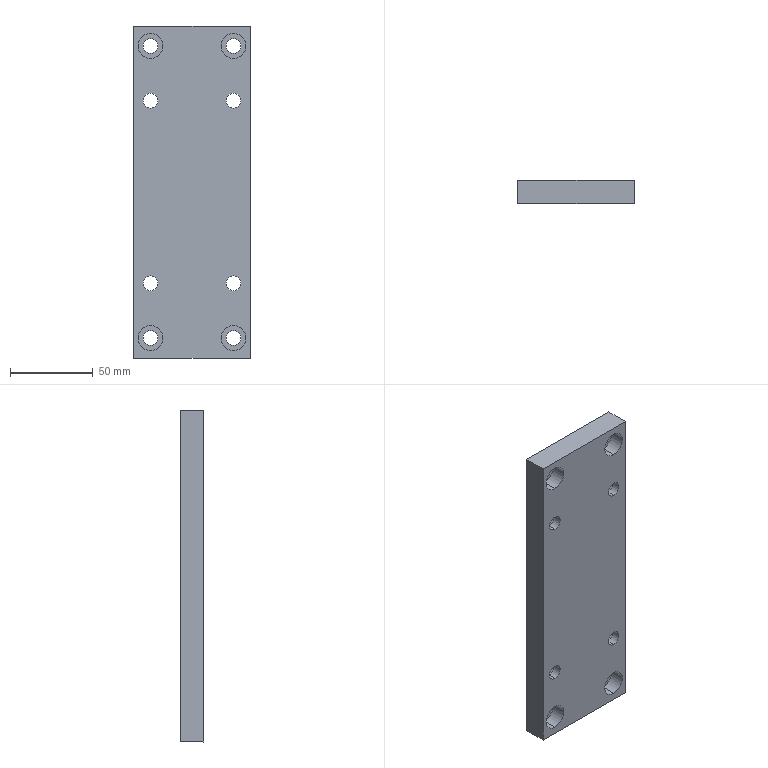Part | SolidWorks | features HoleWzd 2, Extrusion 1 | 1 solid | 46 faces | box 70 x 14 x 200 mm | volume 180732 mm3 | cylinder 32 | plane 14 | commonest cylinder face diameters 9 x16 15 x16
STEP:
#1=CARTESIAN_POINT('',(60.,9.,-180.5));
#2=VERTEX_POINT('',#1);
#3=CARTESIAN_POINT('',(60.,9.,-195.5));
#4=VERTEX_POINT('',#3);
#5=CARTESIAN_POINT('',(60.,9.,-188.));
#6=DIRECTION('',(0.,-1.,0.));
#7=DIRECTION('',(0.,0.,-1.));
#8=AXIS2_PLACEMENT_3D('',#5,#6,#7);
#9=CIRCLE('',#8,7.5);
#10=EDGE_CURVE('',#2,#4,#9,.T.);
#11=ORIENTED_EDGE('',*,*,#10,.F.);
#12=CARTESIAN_POINT('',(60.,0.,-180.5));
#13=VERTEX_POINT('',#12);
#14=CARTESIAN_POINT('',(60.,0.,-180.5));
#15=DIRECTION('',(0.,-1.,0.));
#16=VECTOR('',#15,1000.);
#17=LINE('',#14,#16);
#18=EDGE_CURVE('',#2,#13,#17,.T.);
#19=ORIENTED_EDGE('',*,*,#18,.T.);
#20=CARTESIAN_POINT('',(60.,0.,-195.5));
#21=VERTEX_POINT('',#20);
#22=CARTESIAN_POINT('',(60.,0.,-188.));
#23=DIRECTION('',(0.,-1.,0.));
#24=DIRECTION('',(0.,0.,-1.));
#25=AXIS2_PLACEMENT_3D('',#22,#23,#24);
#26=CIRCLE('',#25,7.5);
#27=EDGE_CURVE('',#13,#21,#26,.T.);
#28=ORIENTED_EDGE('',*,*,#27,.T.);
#29=CARTESIAN_POINT('',(60.,0.,-195.5));
#30=DIRECTION('',(0.,-1.,0.));
#31=VECTOR('',#30,1000.);
#32=LINE('',#29,#31);
#33=EDGE_CURVE('',#4,#21,#32,.T.);
#34=ORIENTED_EDGE('',*,*,#33,.F.);
#35=EDGE_LOOP('',(#11,#19,#28,#34));
#36=FACE_OUTER_BOUND('',#35,.T.);
#37=CARTESIAN_POINT('',(60.,0.,-188.));
#38=DIRECTION('',(0.,-1.,0.));
#39=DIRECTION('',(0.,0.,-1.));
#40=AXIS2_PLACEMENT_3D('',#37,#38,#39);
#41=CYLINDRICAL_SURFACE('',#40,7.5);
#42=ADVANCED_FACE('',(#36),#41,.F.);
#43=CARTESIAN_POINT('',(60.,14.,-183.5));
#44=VERTEX_POINT('',#43);
#45=CARTESIAN_POINT('',(60.,14.,-192.5));
#46=VERTEX_POINT('',#45);
#47=CARTESIAN_POINT('',(60.,14.,-188.));
#48=DIRECTION('',(0.,-1.,0.));
#49=DIRECTION('',(0.,0.,-1.));
#50=AXIS2_PLACEMENT_3D('',#47,#48,#49);
#51=CIRCLE('',#50,4.5);
#52=EDGE_CURVE('',#44,#46,#51,.T.);
#53=ORIENTED_EDGE('',*,*,#52,.F.);
#54=CARTESIAN_POINT('',(60.,9.,-183.5));
#55=VERTEX_POINT('',#54);
#56=CARTESIAN_POINT('',(60.,0.,-183.5));
#57=DIRECTION('',(0.,-1.,0.));
#58=VECTOR('',#57,1000.);
#59=LINE('',#56,#58);
#60=EDGE_CURVE('',#44,#55,#59,.T.);
#61=ORIENTED_EDGE('',*,*,#60,.T.);
#62=CARTESIAN_POINT('',(60.,9.,-192.5));
#63=VERTEX_POINT('',#62);
#64=CARTESIAN_POINT('',(60.,9.,-188.));
#65=DIRECTION('',(0.,-1.,0.));
#66=DIRECTION('',(0.,0.,-1.));
#67=AXIS2_PLACEMENT_3D('',#64,#65,#66);
#68=CIRCLE('',#67,4.5);
#69=EDGE_CURVE('',#55,#63,#68,.T.);
#70=ORIENTED_EDGE('',*,*,#69,.T.);
#71=CARTESIAN_POINT('',(60.,0.,-192.5));
#72=DIRECTION('',(0.,-1.,0.));
#73=VECTOR('',#72,1000.);
#74=LINE('',#71,#73);
#75=EDGE_CURVE('',#46,#63,#74,.T.);
#76=ORIENTED_EDGE('',*,*,#75,.F.);
#77=EDGE_LOOP('',(#53,#61,#70,#76));
#78=FACE_OUTER_BOUND('',#77,.T.);
#79=CARTESIAN_POINT('',(60.,0.,-188.));
#80=DIRECTION('',(0.,-1.,0.));
#81=DIRECTION('',(0.,0.,-1.));
#82=AXIS2_PLACEMENT_3D('',#79,#80,#81);
#83=CYLINDRICAL_SURFACE('',#82,4.5);
#84=ADVANCED_FACE('',(#78),#83,.F.);
#85=CARTESIAN_POINT('',(10.,9.,-180.5));
#86=VERTEX_POINT('',#85);
#87=CARTESIAN_POINT('',(10.,9.,-195.5));
#88=VERTEX_POINT('',#87);
#89=CARTESIAN_POINT('',(10.,9.,-188.));
#90=DIRECTION('',(0.,-1.,0.));
#91=DIRECTION('',(0.,0.,-1.));
#92=AXIS2_PLACEMENT_3D('',#89,#90,#91);
#93=CIRCLE('',#92,7.5);
#94=EDGE_CURVE('',#86,#88,#93,.T.);
#95=ORIENTED_EDGE('',*,*,#94,.F.);
#96=CARTESIAN_POINT('',(10.,0.,-180.5));
#97=VERTEX_POINT('',#96);
#98=CARTESIAN_POINT('',(10.,0.,-180.5));
#99=DIRECTION('',(0.,-1.,0.));
#100=VECTOR('',#99,1000.);
#101=LINE('',#98,#100);
#102=EDGE_CURVE('',#86,#97,#101,.T.);
#103=ORIENTED_EDGE('',*,*,#102,.T.);
#104=CARTESIAN_POINT('',(10.,0.,-195.5));
#105=VERTEX_POINT('',#104);
#106=CARTESIAN_POINT('',(10.,0.,-188.));
#107=DIRECTION('',(0.,-1.,0.));
#108=DIRECTION('',(0.,0.,-1.));
#109=AXIS2_PLACEMENT_3D('',#106,#107,#108);
#110=CIRCLE('',#109,7.5);
#111=EDGE_CURVE('',#97,#105,#110,.T.);
#112=ORIENTED_EDGE('',*,*,#111,.T.);
#113=CARTESIAN_POINT('',(10.,0.,-195.5));
#114=DIRECTION('',(0.,-1.,0.));
#115=VECTOR('',#114,1000.);
#116=LINE('',#113,#115);
#117=EDGE_CURVE('',#88,#105,#116,.T.);
#118=ORIENTED_EDGE('',*,*,#117,.F.);
#119=EDGE_LOOP('',(#95,#103,#112,#118));
#120=FACE_OUTER_BOUND('',#119,.T.);
#121=CARTESIAN_POINT('',(10.,0.,-188.));
#122=DIRECTION('',(0.,-1.,0.));
#123=DIRECTION('',(0.,0.,-1.));
#124=AXIS2_PLACEMENT_3D('',#121,#122,#123);
#125=CYLINDRICAL_SURFACE('',#124,7.5);
#126=ADVANCED_FACE('',(#120),#125,.F.);
#127=CARTESIAN_POINT('',(10.,14.,-183.5));
#128=VERTEX_POINT('',#127);
#129=CARTESIAN_POINT('',(10.,14.,-192.5));
#130=VERTEX_POINT('',#129);
#131=CARTESIAN_POINT('',(10.,14.,-188.));
#132=DIRECTION('',(0.,-1.,0.));
#133=DIRECTION('',(0.,0.,-1.));
#134=AXIS2_PLACEMENT_3D('',#131,#132,#133);
#135=CIRCLE('',#134,4.5);
#136=EDGE_CURVE('',#128,#130,#135,.T.);
#137=ORIENTED_EDGE('',*,*,#136,.F.);
#138=CARTESIAN_POINT('',(10.,9.,-183.5));
#139=VERTEX_POINT('',#138);
#140=CARTESIAN_POINT('',(10.,0.,-183.5));
#141=DIRECTION('',(0.,-1.,0.));
#142=VECTOR('',#141,1000.);
#143=LINE('',#140,#142);
#144=EDGE_CURVE('',#128,#139,#143,.T.);
#145=ORIENTED_EDGE('',*,*,#144,.T.);
#146=CARTESIAN_POINT('',(10.,9.,-192.5));
#147=VERTEX_POINT('',#146);
#148=CARTESIAN_POINT('',(10.,9.,-188.));
#149=DIRECTION('',(0.,-1.,0.));
#150=DIRECTION('',(0.,0.,-1.));
#151=AXIS2_PLACEMENT_3D('',#148,#149,#150);
#152=CIRCLE('',#151,4.5);
#153=EDGE_CURVE('',#139,#147,#152,.T.);
#154=ORIENTED_EDGE('',*,*,#153,.T.);
#155=CARTESIAN_POINT('',(10.,0.,-192.5));
#156=DIRECTION('',(0.,-1.,0.));
#157=VECTOR('',#156,1000.);
#158=LINE('',#155,#157);
#159=EDGE_CURVE('',#130,#147,#158,.T.);
#160=ORIENTED_EDGE('',*,*,#159,.F.);
#161=EDGE_LOOP('',(#137,#145,#154,#160));
#162=FACE_OUTER_BOUND('',#161,.T.);
#163=CARTESIAN_POINT('',(10.,0.,-188.));
#164=DIRECTION('',(0.,-1.,0.));
#165=DIRECTION('',(0.,0.,-1.));
#166=AXIS2_PLACEMENT_3D('',#163,#164,#165);
#167=CYLINDRICAL_SURFACE('',#166,4.5);
#168=ADVANCED_FACE('',(#162),#167,.F.);
#169=CARTESIAN_POINT('',(10.,9.,-4.5));
#170=VERTEX_POINT('',#169);
#171=CARTESIAN_POINT('',(10.,9.,-19.5));
#172=VERTEX_POINT('',#171);
#173=CARTESIAN_POINT('',(10.,9.,-12.));
#174=DIRECTION('',(0.,-1.,0.));
#175=DIRECTION('',(0.,0.,-1.));
#176=AXIS2_PLACEMENT_3D('',#173,#174,#175);
#177=CIRCLE('',#176,7.5);
#178=EDGE_CURVE('',#170,#172,#177,.T.);
#179=ORIENTED_EDGE('',*,*,#178,.F.);
#180=CARTESIAN_POINT('',(10.,0.,-4.5));
#181=VERTEX_POINT('',#180);
#182=CARTESIAN_POINT('',(10.,0.,-4.5));
#183=DIRECTION('',(0.,-1.,0.));
#184=VECTOR('',#183,1000.);
#185=LINE('',#182,#184);
#186=EDGE_CURVE('',#170,#181,#185,.T.);
#187=ORIENTED_EDGE('',*,*,#186,.T.);
#188=CARTESIAN_POINT('',(10.,0.,-19.5));
#189=VERTEX_POINT('',#188);
#190=CARTESIAN_POINT('',(10.,0.,-12.));
#191=DIRECTION('',(0.,-1.,0.));
#192=DIRECTION('',(0.,0.,-1.));
#193=AXIS2_PLACEMENT_3D('',#190,#191,#192);
#194=CIRCLE('',#193,7.5);
#195=EDGE_CURVE('',#181,#189,#194,.T.);
#196=ORIENTED_EDGE('',*,*,#195,.T.);
#197=CARTESIAN_POINT('',(10.,0.,-19.5));
#198=DIRECTION('',(0.,-1.,0.));
#199=VECTOR('',#198,1000.);
#200=LINE('',#197,#199);
#201=EDGE_CURVE('',#172,#189,#200,.T.);
#202=ORIENTED_EDGE('',*,*,#201,.F.);
#203=EDGE_LOOP('',(#179,#187,#196,#202));
#204=FACE_OUTER_BOUND('',#203,.T.);
#205=CARTESIAN_POINT('',(10.,0.,-12.));
#206=DIRECTION('',(0.,-1.,0.));
#207=DIRECTION('',(0.,0.,-1.));
#208=AXIS2_PLACEMENT_3D('',#205,#206,#207);
#209=CYLINDRICAL_SURFACE('',#208,7.5);
#210=ADVANCED_FACE('',(#204),#209,.F.);
#211=CARTESIAN_POINT('',(10.,14.,-7.5));
#212=VERTEX_POINT('',#211);
#213=CARTESIAN_POINT('',(10.,14.,-16.5));
#214=VERTEX_POINT('',#213);
#215=CARTESIAN_POINT('',(10.,14.,-12.));
#216=DIRECTION('',(0.,-1.,0.));
#217=DIRECTION('',(0.,0.,-1.));
#218=AXIS2_PLACEMENT_3D('',#215,#216,#217);
#219=CIRCLE('',#218,4.5);
#220=EDGE_CURVE('',#212,#214,#219,.T.);
#221=ORIENTED_EDGE('',*,*,#220,.F.);
#222=CARTESIAN_POINT('',(10.,9.,-7.5));
#223=VERTEX_POINT('',#222);
#224=CARTESIAN_POINT('',(10.,0.,-7.5));
#225=DIRECTION('',(0.,-1.,0.));
#226=VECTOR('',#225,1000.);
#227=LINE('',#224,#226);
#228=EDGE_CURVE('',#212,#223,#227,.T.);
#229=ORIENTED_EDGE('',*,*,#228,.T.);
#230=CARTESIAN_POINT('',(10.,9.,-16.5));
#231=VERTEX_POINT('',#230);
#232=CARTESIAN_POINT('',(10.,9.,-12.));
#233=DIRECTION('',(0.,-1.,0.));
#234=DIRECTION('',(0.,0.,-1.));
#235=AXIS2_PLACEMENT_3D('',#232,#233,#234);
#236=CIRCLE('',#235,4.5);
#237=EDGE_CURVE('',#223,#231,#236,.T.);
#238=ORIENTED_EDGE('',*,*,#237,.T.);
#239=CARTESIAN_POINT('',(10.,0.,-16.5));
#240=DIRECTION('',(0.,-1.,0.));
#241=VECTOR('',#240,1000.);
#242=LINE('',#239,#241);
#243=EDGE_CURVE('',#214,#231,#242,.T.);
#244=ORIENTED_EDGE('',*,*,#243,.F.);
#245=EDGE_LOOP('',(#221,#229,#238,#244));
#246=FACE_OUTER_BOUND('',#245,.T.);
#247=CARTESIAN_POINT('',(10.,0.,-12.));
#248=DIRECTION('',(0.,-1.,0.));
#249=DIRECTION('',(0.,0.,-1.));
#250=AXIS2_PLACEMENT_3D('',#247,#248,#249);
#251=CYLINDRICAL_SURFACE('',#250,4.5);
#252=ADVANCED_FACE('',(#246),#251,.F.);
#253=CARTESIAN_POINT('',(60.,9.,-4.5));
#254=VERTEX_POINT('',#253);
#255=CARTESIAN_POINT('',(60.,9.,-19.5));
#256=VERTEX_POINT('',#255);
#257=CARTESIAN_POINT('',(60.,9.,-12.));
#258=DIRECTION('',(0.,-1.,0.));
#259=DIRECTION('',(0.,0.,-1.));
#260=AXIS2_PLACEMENT_3D('',#257,#258,#259);
#261=CIRCLE('',#260,7.5);
#262=EDGE_CURVE('',#254,#256,#261,.T.);
#263=ORIENTED_EDGE('',*,*,#262,.F.);
#264=CARTESIAN_POINT('',(60.,0.,-4.5));
#265=VERTEX_POINT('',#264);
#266=CARTESIAN_POINT('',(60.,0.,-4.5));
#267=DIRECTION('',(0.,-1.,0.));
#268=VECTOR('',#267,1000.);
#269=LINE('',#266,#268);
#270=EDGE_CURVE('',#254,#265,#269,.T.);
#271=ORIENTED_EDGE('',*,*,#270,.T.);
#272=CARTESIAN_POINT('',(60.,0.,-19.5));
#273=VERTEX_POINT('',#272);
#274=CARTESIAN_POINT('',(60.,0.,-12.));
#275=DIRECTION('',(0.,-1.,0.));
#276=DIRECTION('',(0.,0.,-1.));
#277=AXIS2_PLACEMENT_3D('',#274,#275,#276);
#278=CIRCLE('',#277,7.5);
#279=EDGE_CURVE('',#265,#273,#278,.T.);
#280=ORIENTED_EDGE('',*,*,#279,.T.);
#281=CARTESIAN_POINT('',(60.,0.,-19.5));
#282=DIRECTION('',(0.,-1.,0.));
#283=VECTOR('',#282,1000.);
#284=LINE('',#281,#283);
#285=EDGE_CURVE('',#256,#273,#284,.T.);
#286=ORIENTED_EDGE('',*,*,#285,.F.);
#287=EDGE_LOOP('',(#263,#271,#280,#286));
#288=FACE_OUTER_BOUND('',#287,.T.);
#289=CARTESIAN_POINT('',(60.,0.,-12.));
#290=DIRECTION('',(0.,-1.,0.));
#291=DIRECTION('',(0.,0.,-1.));
#292=AXIS2_PLACEMENT_3D('',#289,#290,#291);
#293=CYLINDRICAL_SURFACE('',#292,7.5);
#294=ADVANCED_FACE('',(#288),#293,.F.);
#295=CARTESIAN_POINT('',(60.,14.,-7.5));
#296=VERTEX_POINT('',#295);
#297=CARTESIAN_POINT('',(60.,14.,-16.5));
#298=VERTEX_POINT('',#297);
#299=CARTESIAN_POINT('',(60.,14.,-12.));
#300=DIRECTION('',(0.,-1.,0.));
#301=DIRECTION('',(0.,0.,-1.));
#302=AXIS2_PLACEMENT_3D('',#299,#300,#301);
#303=CIRCLE('',#302,4.5);
#304=EDGE_CURVE('',#296,#298,#303,.T.);
#305=ORIENTED_EDGE('',*,*,#304,.F.);
#306=CARTESIAN_POINT('',(60.,9.,-7.5));
#307=VERTEX_POINT('',#306);
#308=CARTESIAN_POINT('',(60.,0.,-7.5));
#309=DIRECTION('',(0.,-1.,0.));
#310=VECTOR('',#309,1000.);
#311=LINE('',#308,#310);
#312=EDGE_CURVE('',#296,#307,#311,.T.);
#313=ORIENTED_EDGE('',*,*,#312,.T.);
#314=CARTESIAN_POINT('',(60.,9.,-16.5));
#315=VERTEX_POINT('',#314);
#316=CARTESIAN_POINT('',(60.,9.,-12.));
#317=DIRECTION('',(0.,-1.,0.));
#318=DIRECTION('',(0.,0.,-1.));
#319=AXIS2_PLACEMENT_3D('',#316,#317,#318);
#320=CIRCLE('',#319,4.5);
#321=EDGE_CURVE('',#307,#315,#320,.T.);
#322=ORIENTED_EDGE('',*,*,#321,.T.);
#323=CARTESIAN_POINT('',(60.,0.,-16.5));
#324=DIRECTION('',(0.,-1.,0.));
#325=VECTOR('',#324,1000.);
#326=LINE('',#323,#325);
#327=EDGE_CURVE('',#298,#315,#326,.T.);
#328=ORIENTED_EDGE('',*,*,#327,.F.);
#329=EDGE_LOOP('',(#305,#313,#322,#328));
#330=FACE_OUTER_BOUND('',#329,.T.);
#331=CARTESIAN_POINT('',(60.,0.,-12.));
#332=DIRECTION('',(0.,-1.,0.));
#333=DIRECTION('',(0.,0.,-1.));
#334=AXIS2_PLACEMENT_3D('',#331,#332,#333);
#335=CYLINDRICAL_SURFACE('',#334,4.5);
#336=ADVANCED_FACE('',(#330),#335,.F.);
#337=CARTESIAN_POINT('',(10.,5.,-162.5));
#338=VERTEX_POINT('',#337);
#339=CARTESIAN_POINT('',(10.,5.,-147.5));
#340=VERTEX_POINT('',#339);
#341=CARTESIAN_POINT('',(10.,5.,-155.));
#342=DIRECTION('',(0.,1.,0.));
#343=DIRECTION('',(0.,0.,1.));
#344=AXIS2_PLACEMENT_3D('',#341,#342,#343);
#345=CIRCLE('',#344,7.5);
#346=EDGE_CURVE('',#338,#340,#345,.T.);
#347=ORIENTED_EDGE('',*,*,#346,.F.);
#348=CARTESIAN_POINT('',(10.,14.,-162.5));
#349=VERTEX_POINT('',#348);
#350=CARTESIAN_POINT('',(10.,14.,-162.5));
#351=DIRECTION('',(0.,1.,0.));
#352=VECTOR('',#351,1000.);
#353=LINE('',#350,#352);
#354=EDGE_CURVE('',#338,#349,#353,.T.);
#355=ORIENTED_EDGE('',*,*,#354,.T.);
#356=CARTESIAN_POINT('',(10.,14.,-147.5));
#357=VERTEX_POINT('',#356);
#358=CARTESIAN_POINT('',(10.,14.,-155.));
#359=DIRECTION('',(0.,1.,0.));
#360=DIRECTION('',(0.,0.,1.));
#361=AXIS2_PLACEMENT_3D('',#358,#359,#360);
#362=CIRCLE('',#361,7.5);
#363=EDGE_CURVE('',#349,#357,#362,.T.);
#364=ORIENTED_EDGE('',*,*,#363,.T.);
#365=CARTESIAN_POINT('',(10.,14.,-147.5));
#366=DIRECTION('',(0.,1.,0.));
#367=VECTOR('',#366,1000.);
#368=LINE('',#365,#367);
#369=EDGE_CURVE('',#340,#357,#368,.T.);
#370=ORIENTED_EDGE('',*,*,#369,.F.);
#371=EDGE_LOOP('',(#347,#355,#364,#370));
#372=FACE_OUTER_BOUND('',#371,.T.);
#373=CARTESIAN_POINT('',(10.,14.,-155.));
#374=DIRECTION('',(0.,1.,0.));
#375=DIRECTION('',(0.,0.,1.));
#376=AXIS2_PLACEMENT_3D('',#373,#374,#375);
#377=CYLINDRICAL_SURFACE('',#376,7.5);
#378=ADVANCED_FACE('',(#372),#377,.F.);
#379=CARTESIAN_POINT('',(10.,0.,-159.5));
#380=VERTEX_POINT('',#379);
#381=CARTESIAN_POINT('',(10.,0.,-150.5));
#382=VERTEX_POINT('',#381);
#383=CARTESIAN_POINT('',(10.,0.,-155.));
#384=DIRECTION('',(0.,1.,0.));
#385=DIRECTION('',(0.,0.,1.));
#386=AXIS2_PLACEMENT_3D('',#383,#384,#385);
#387=CIRCLE('',#386,4.5);
#388=EDGE_CURVE('',#380,#382,#387,.T.);
#389=ORIENTED_EDGE('',*,*,#388,.F.);
#390=CARTESIAN_POINT('',(10.,5.,-159.5));
#391=VERTEX_POINT('',#390);
#392=CARTESIAN_POINT('',(10.,14.,-159.5));
#393=DIRECTION('',(0.,1.,0.));
#394=VECTOR('',#393,1000.);
#395=LINE('',#392,#394);
#396=EDGE_CURVE('',#380,#391,#395,.T.);
#397=ORIENTED_EDGE('',*,*,#396,.T.);
#398=CARTESIAN_POINT('',(10.,5.,-150.5));
#399=VERTEX_POINT('',#398);
#400=CARTESIAN_POINT('',(10.,5.,-155.));
#401=DIRECTION('',(0.,1.,0.));
#402=DIRECTION('',(0.,0.,1.));
#403=AXIS2_PLACEMENT_3D('',#400,#401,#402);
#404=CIRCLE('',#403,4.5);
#405=EDGE_CURVE('',#391,#399,#404,.T.);
#406=ORIENTED_EDGE('',*,*,#405,.T.);
#407=CARTESIAN_POINT('',(10.,14.,-150.5));
#408=DIRECTION('',(0.,1.,0.));
#409=VECTOR('',#408,1000.);
#410=LINE('',#407,#409);
#411=EDGE_CURVE('',#382,#399,#410,.T.);
#412=ORIENTED_EDGE('',*,*,#411,.F.);
#413=EDGE_LOOP('',(#389,#397,#406,#412));
#414=FACE_OUTER_BOUND('',#413,.T.);
#415=CARTESIAN_POINT('',(10.,14.,-155.));
#416=DIRECTION('',(0.,1.,0.));
#417=DIRECTION('',(0.,0.,1.));
#418=AXIS2_PLACEMENT_3D('',#415,#416,#417);
#419=CYLINDRICAL_SURFACE('',#418,4.5);
#420=ADVANCED_FACE('',(#414),#419,.F.);
#421=CARTESIAN_POINT('',(60.,5.,-162.5));
#422=VERTEX_POINT('',#421);
#423=CARTESIAN_POINT('',(60.,5.,-147.5));
#424=VERTEX_POINT('',#423);
#425=CARTESIAN_POINT('',(60.,5.,-155.));
#426=DIRECTION('',(0.,1.,0.));
#427=DIRECTION('',(0.,0.,1.));
#428=AXIS2_PLACEMENT_3D('',#425,#426,#427);
#429=CIRCLE('',#428,7.5);
#430=EDGE_CURVE('',#422,#424,#429,.T.);
#431=ORIENTED_EDGE('',*,*,#430,.F.);
#432=CARTESIAN_POINT('',(60.,14.,-162.5));
#433=VERTEX_POINT('',#432);
#434=CARTESIAN_POINT('',(60.,14.,-162.5));
#435=DIRECTION('',(0.,1.,0.));
#436=VECTOR('',#435,1000.);
#437=LINE('',#434,#436);
#438=EDGE_CURVE('',#422,#433,#437,.T.);
#439=ORIENTED_EDGE('',*,*,#438,.T.);
#440=CARTESIAN_POINT('',(60.,14.,-147.5));
#441=VERTEX_POINT('',#440);
#442=CARTESIAN_POINT('',(60.,14.,-155.));
#443=DIRECTION('',(0.,1.,0.));
#444=DIRECTION('',(0.,0.,1.));
#445=AXIS2_PLACEMENT_3D('',#442,#443,#444);
#446=CIRCLE('',#445,7.5);
#447=EDGE_CURVE('',#433,#441,#446,.T.);
#448=ORIENTED_EDGE('',*,*,#447,.T.);
#449=CARTESIAN_POINT('',(60.,14.,-147.5));
#450=DIRECTION('',(0.,1.,0.));
#451=VECTOR('',#450,1000.);
#452=LINE('',#449,#451);
#453=EDGE_CURVE('',#424,#441,#452,.T.);
#454=ORIENTED_EDGE('',*,*,#453,.F.);
#455=EDGE_LOOP('',(#431,#439,#448,#454));
#456=FACE_OUTER_BOUND('',#455,.T.);
#457=CARTESIAN_POINT('',(60.,14.,-155.));
#458=DIRECTION('',(0.,1.,0.));
#459=DIRECTION('',(0.,0.,1.));
#460=AXIS2_PLACEMENT_3D('',#457,#458,#459);
#461=CYLINDRICAL_SURFACE('',#460,7.5);
#462=ADVANCED_FACE('',(#456),#461,.F.);
#463=CARTESIAN_POINT('',(60.,0.,-159.5));
#464=VERTEX_POINT('',#463);
#465=CARTESIAN_POINT('',(60.,0.,-150.5));
#466=VERTEX_POINT('',#465);
#467=CARTESIAN_POINT('',(60.,0.,-155.));
#468=DIRECTION('',(0.,1.,0.));
#469=DIRECTION('',(0.,0.,1.));
#470=AXIS2_PLACEMENT_3D('',#467,#468,#469);
#471=CIRCLE('',#470,4.5);
#472=EDGE_CURVE('',#464,#466,#471,.T.);
#473=ORIENTED_EDGE('',*,*,#472,.F.);
#474=CARTESIAN_POINT('',(60.,5.,-159.5));
#475=VERTEX_POINT('',#474);
#476=CARTESIAN_POINT('',(60.,14.,-159.5));
#477=DIRECTION('',(0.,1.,0.));
#478=VECTOR('',#477,1000.);
#479=LINE('',#476,#478);
#480=EDGE_CURVE('',#464,#475,#479,.T.);
#481=ORIENTED_EDGE('',*,*,#480,.T.);
#482=CARTESIAN_POINT('',(60.,5.,-150.5));
#483=VERTEX_POINT('',#482);
#484=CARTESIAN_POINT('',(60.,5.,-155.));
#485=DIRECTION('',(0.,1.,0.));
#486=DIRECTION('',(0.,0.,1.));
#487=AXIS2_PLACEMENT_3D('',#484,#485,#486);
#488=CIRCLE('',#487,4.5);
#489=EDGE_CURVE('',#475,#483,#488,.T.);
#490=ORIENTED_EDGE('',*,*,#489,.T.);
#491=CARTESIAN_POINT('',(60.,14.,-150.5));
#492=DIRECTION('',(0.,1.,0.));
#493=VECTOR('',#492,1000.);
#494=LINE('',#491,#493);
#495=EDGE_CURVE('',#466,#483,#494,.T.);
#496=ORIENTED_EDGE('',*,*,#495,.F.);
#497=EDGE_LOOP('',(#473,#481,#490,#496));
#498=FACE_OUTER_BOUND('',#497,.T.);
#499=CARTESIAN_POINT('',(60.,14.,-155.));
#500=DIRECTION('',(0.,1.,0.));
#501=DIRECTION('',(0.,0.,1.));
#502=AXIS2_PLACEMENT_3D('',#499,#500,#501);
#503=CYLINDRICAL_SURFACE('',#502,4.5);
#504=ADVANCED_FACE('',(#498),#503,.F.);
#505=CARTESIAN_POINT('',(60.,5.,-52.5));
#506=VERTEX_POINT('',#505);
#507=CARTESIAN_POINT('',(60.,5.,-37.5));
#508=VERTEX_POINT('',#507);
#509=CARTESIAN_POINT('',(60.,5.,-45.));
#510=DIRECTION('',(0.,1.,0.));
#511=DIRECTION('',(0.,0.,1.));
#512=AXIS2_PLACEMENT_3D('',#509,#510,#511);
#513=CIRCLE('',#512,7.5);
#514=EDGE_CURVE('',#506,#508,#513,.T.);
#515=ORIENTED_EDGE('',*,*,#514,.F.);
#516=CARTESIAN_POINT('',(60.,14.,-52.5));
#517=VERTEX_POINT('',#516);
#518=CARTESIAN_POINT('',(60.,14.,-52.5));
#519=DIRECTION('',(0.,1.,0.));
#520=VECTOR('',#519,1000.);
#521=LINE('',#518,#520);
#522=EDGE_CURVE('',#506,#517,#521,.T.);
#523=ORIENTED_EDGE('',*,*,#522,.T.);
#524=CARTESIAN_POINT('',(60.,14.,-37.5));
#525=VERTEX_POINT('',#524);
#526=CARTESIAN_POINT('',(60.,14.,-45.));
#527=DIRECTION('',(0.,1.,0.));
#528=DIRECTION('',(0.,0.,1.));
#529=AXIS2_PLACEMENT_3D('',#526,#527,#528);
#530=CIRCLE('',#529,7.5);
#531=EDGE_CURVE('',#517,#525,#530,.T.);
#532=ORIENTED_EDGE('',*,*,#531,.T.);
#533=CARTESIAN_POINT('',(60.,14.,-37.5));
#534=DIRECTION('',(0.,1.,0.));
#535=VECTOR('',#534,1000.);
#536=LINE('',#533,#535);
#537=EDGE_CURVE('',#508,#525,#536,.T.);
#538=ORIENTED_EDGE('',*,*,#537,.F.);
#539=EDGE_LOOP('',(#515,#523,#532,#538));
#540=FACE_OUTER_BOUND('',#539,.T.);
#541=CARTESIAN_POINT('',(60.,14.,-45.));
#542=DIRECTION('',(0.,1.,0.));
#543=DIRECTION('',(0.,0.,1.));
#544=AXIS2_PLACEMENT_3D('',#541,#542,#543);
#545=CYLINDRICAL_SURFACE('',#544,7.5);
#546=ADVANCED_FACE('',(#540),#545,.F.);
#547=CARTESIAN_POINT('',(60.,0.,-49.5));
#548=VERTEX_POINT('',#547);
#549=CARTESIAN_POINT('',(60.,0.,-40.5));
#550=VERTEX_POINT('',#549);
#551=CARTESIAN_POINT('',(60.,0.,-45.));
#552=DIRECTION('',(0.,1.,0.));
#553=DIRECTION('',(0.,0.,1.));
#554=AXIS2_PLACEMENT_3D('',#551,#552,#553);
#555=CIRCLE('',#554,4.5);
#556=EDGE_CURVE('',#548,#550,#555,.T.);
#557=ORIENTED_EDGE('',*,*,#556,.F.);
#558=CARTESIAN_POINT('',(60.,5.,-49.5));
#559=VERTEX_POINT('',#558);
#560=CARTESIAN_POINT('',(60.,14.,-49.5));
#561=DIRECTION('',(0.,1.,0.));
#562=VECTOR('',#561,1000.);
#563=LINE('',#560,#562);
#564=EDGE_CURVE('',#548,#559,#563,.T.);
#565=ORIENTED_EDGE('',*,*,#564,.T.);
#566=CARTESIAN_POINT('',(60.,5.,-40.5));
#567=VERTEX_POINT('',#566);
#568=CARTESIAN_POINT('',(60.,5.,-45.));
#569=DIRECTION('',(0.,1.,0.));
#570=DIRECTION('',(0.,0.,1.));
#571=AXIS2_PLACEMENT_3D('',#568,#569,#570);
#572=CIRCLE('',#571,4.5);
#573=EDGE_CURVE('',#559,#567,#572,.T.);
#574=ORIENTED_EDGE('',*,*,#573,.T.);
#575=CARTESIAN_POINT('',(60.,14.,-40.5));
#576=DIRECTION('',(0.,1.,0.));
#577=VECTOR('',#576,1000.);
#578=LINE('',#575,#577);
#579=EDGE_CURVE('',#550,#567,#578,.T.);
#580=ORIENTED_EDGE('',*,*,#579,.F.);
#581=EDGE_LOOP('',(#557,#565,#574,#580));
#582=FACE_OUTER_BOUND('',#581,.T.);
#583=CARTESIAN_POINT('',(60.,14.,-45.));
#584=DIRECTION('',(0.,1.,0.));
#585=DIRECTION('',(0.,0.,1.));
#586=AXIS2_PLACEMENT_3D('',#583,#584,#585);
#587=CYLINDRICAL_SURFACE('',#586,4.5);
#588=ADVANCED_FACE('',(#582),#587,.F.);
#589=CARTESIAN_POINT('',(10.,5.,-52.5));
#590=VERTEX_POINT('',#589);
#591=CARTESIAN_POINT('',(10.,5.,-37.5));
#592=VERTEX_POINT('',#591);
#593=CARTESIAN_POINT('',(10.,5.,-45.));
#594=DIRECTION('',(0.,1.,0.));
#595=DIRECTION('',(0.,0.,1.));
#596=AXIS2_PLACEMENT_3D('',#593,#594,#595);
#597=CIRCLE('',#596,7.5);
#598=EDGE_CURVE('',#590,#592,#597,.T.);
#599=ORIENTED_EDGE('',*,*,#598,.F.);
#600=CARTESIAN_POINT('',(10.,14.,-52.5));
#601=VERTEX_POINT('',#600);
#602=CARTESIAN_POINT('',(10.,14.,-52.5));
#603=DIRECTION('',(0.,1.,0.));
#604=VECTOR('',#603,1000.);
#605=LINE('',#602,#604);
#606=EDGE_CURVE('',#590,#601,#605,.T.);
#607=ORIENTED_EDGE('',*,*,#606,.T.);
#608=CARTESIAN_POINT('',(10.,14.,-37.5));
#609=VERTEX_POINT('',#608);
#610=CARTESIAN_POINT('',(10.,14.,-45.));
#611=DIRECTION('',(0.,1.,0.));
#612=DIRECTION('',(0.,0.,1.));
#613=AXIS2_PLACEMENT_3D('',#610,#611,#612);
#614=CIRCLE('',#613,7.5);
#615=EDGE_CURVE('',#601,#609,#614,.T.);
#616=ORIENTED_EDGE('',*,*,#615,.T.);
#617=CARTESIAN_POINT('',(10.,14.,-37.5));
#618=DIRECTION('',(0.,1.,0.));
#619=VECTOR('',#618,1000.);
#620=LINE('',#617,#619);
#621=EDGE_CURVE('',#592,#609,#620,.T.);
#622=ORIENTED_EDGE('',*,*,#621,.F.);
#623=EDGE_LOOP('',(#599,#607,#616,#622));
#624=FACE_OUTER_BOUND('',#623,.T.);
#625=CARTESIAN_POINT('',(10.,14.,-45.));
#626=DIRECTION('',(0.,1.,0.));
#627=DIRECTION('',(0.,0.,1.));
#628=AXIS2_PLACEMENT_3D('',#625,#626,#627);
#629=CYLINDRICAL_SURFACE('',#628,7.5);
#630=ADVANCED_FACE('',(#624),#629,.F.);
#631=CARTESIAN_POINT('',(10.,0.,-49.5));
#632=VERTEX_POINT('',#631);
#633=CARTESIAN_POINT('',(10.,0.,-40.5));
#634=VERTEX_POINT('',#633);
#635=CARTESIAN_POINT('',(10.,0.,-45.));
#636=DIRECTION('',(0.,1.,0.));
#637=DIRECTION('',(0.,0.,1.));
#638=AXIS2_PLACEMENT_3D('',#635,#636,#637);
#639=CIRCLE('',#638,4.5);
#640=EDGE_CURVE('',#632,#634,#639,.T.);
#641=ORIENTED_EDGE('',*,*,#640,.F.);
#642=CARTESIAN_POINT('',(10.,5.,-49.5));
#643=VERTEX_POINT('',#642);
#644=CARTESIAN_POINT('',(10.,14.,-49.5));
#645=DIRECTION('',(0.,1.,0.));
#646=VECTOR('',#645,1000.);
#647=LINE('',#644,#646);
#648=EDGE_CURVE('',#632,#643,#647,.T.);
#649=ORIENTED_EDGE('',*,*,#648,.T.);
#650=CARTESIAN_POINT('',(10.,5.,-40.5));
#651=VERTEX_POINT('',#650);
#652=CARTESIAN_POINT('',(10.,5.,-45.));
#653=DIRECTION('',(0.,1.,0.));
#654=DIRECTION('',(0.,0.,1.));
#655=AXIS2_PLACEMENT_3D('',#652,#653,#654);
#656=CIRCLE('',#655,4.5);
#657=EDGE_CURVE('',#643,#651,#656,.T.);
#658=ORIENTED_EDGE('',*,*,#657,.T.);
#659=CARTESIAN_POINT('',(10.,14.,-40.5));
#660=DIRECTION('',(0.,1.,0.));
#661=VECTOR('',#660,1000.);
#662=LINE('',#659,#661);
#663=EDGE_CURVE('',#634,#651,#662,.T.);
#664=ORIENTED_EDGE('',*,*,#663,.F.);
#665=EDGE_LOOP('',(#641,#649,#658,#664));
#666=FACE_OUTER_BOUND('',#665,.T.);
#667=CARTESIAN_POINT('',(10.,14.,-45.));
#668=DIRECTION('',(0.,1.,0.));
#669=DIRECTION('',(0.,0.,1.));
#670=AXIS2_PLACEMENT_3D('',#667,#668,#669);
#671=CYLINDRICAL_SURFACE('',#670,4.5);
#672=ADVANCED_FACE('',(#666),#671,.F.);
#673=CARTESIAN_POINT('',(70.,0.,0.));
#674=VERTEX_POINT('',#673);
#675=CARTESIAN_POINT('',(70.,0.,-200.));
#676=VERTEX_POINT('',#675);
#677=CARTESIAN_POINT('',(70.,0.,0.));
#678=DIRECTION('',(0.,0.,-1.));
#679=VECTOR('',#678,1000.);
#680=LINE('',#677,#679);
#681=EDGE_CURVE('',#674,#676,#680,.T.);
#682=ORIENTED_EDGE('',*,*,#681,.T.);
#683=CARTESIAN_POINT('',(70.,14.,-200.));
#684=VERTEX_POINT('',#683);
#685=CARTESIAN_POINT('',(70.,14.,-200.));
#686=DIRECTION('',(0.,-1.,0.));
#687=VECTOR('',#686,1000.);
#688=LINE('',#685,#687);
#689=EDGE_CURVE('',#684,#676,#688,.T.);
#690=ORIENTED_EDGE('',*,*,#689,.F.);
#691=CARTESIAN_POINT('',(70.,14.,0.));
#692=VERTEX_POINT('',#691);
#693=CARTESIAN_POINT('',(70.,14.,0.));
#694=DIRECTION('',(0.,0.,-1.));
#695=VECTOR('',#694,1000.);
#696=LINE('',#693,#695);
#697=EDGE_CURVE('',#692,#684,#696,.T.);
#698=ORIENTED_EDGE('',*,*,#697,.F.);
#699=CARTESIAN_POINT('',(70.,14.,0.));
#700=DIRECTION('',(0.,-1.,0.));
#701=VECTOR('',#700,1000.);
#702=LINE('',#699,#701);
#703=EDGE_CURVE('',#692,#674,#702,.T.);
#704=ORIENTED_EDGE('',*,*,#703,.T.);
#705=EDGE_LOOP('',(#682,#690,#698,#704));
#706=FACE_OUTER_BOUND('',#705,.T.);
#707=CARTESIAN_POINT('',(70.,14.,0.));
#708=DIRECTION('',(-1.,0.,0.));
#709=DIRECTION('',(0.,0.,1.));
#710=AXIS2_PLACEMENT_3D('',#707,#708,#709);
#711=PLANE('',#710);
#712=ADVANCED_FACE('',(#706),#711,.F.);
#713=CARTESIAN_POINT('',(0.,0.,-200.));
#714=VERTEX_POINT('',#713);
#715=CARTESIAN_POINT('',(0.,0.,-200.));
#716=DIRECTION('',(-1.,0.,0.));
#717=VECTOR('',#716,1000.);
#718=LINE('',#715,#717);
#719=EDGE_CURVE('',#676,#714,#718,.T.);
#720=ORIENTED_EDGE('',*,*,#719,.T.);
#721=CARTESIAN_POINT('',(0.,14.,-200.));
#722=VERTEX_POINT('',#721);
#723=CARTESIAN_POINT('',(0.,14.,-200.));
#724=DIRECTION('',(0.,-1.,0.));
#725=VECTOR('',#724,1000.);
#726=LINE('',#723,#725);
#727=EDGE_CURVE('',#722,#714,#726,.T.);
#728=ORIENTED_EDGE('',*,*,#727,.F.);
#729=CARTESIAN_POINT('',(0.,14.,-200.));
#730=DIRECTION('',(-1.,0.,0.));
#731=VECTOR('',#730,1000.);
#732=LINE('',#729,#731);
#733=EDGE_CURVE('',#684,#722,#732,.T.);
#734=ORIENTED_EDGE('',*,*,#733,.F.);
#735=ORIENTED_EDGE('',*,*,#689,.T.);
#736=EDGE_LOOP('',(#720,#728,#734,#735));
#737=FACE_OUTER_BOUND('',#736,.T.);
#738=CARTESIAN_POINT('',(0.,14.,-200.));
#739=DIRECTION('',(0.,0.,1.));
#740=DIRECTION('',(1.,0.,0.));
#741=AXIS2_PLACEMENT_3D('',#738,#739,#740);
#742=PLANE('',#741);
#743=ADVANCED_FACE('',(#737),#742,.F.);
#744=CARTESIAN_POINT('',(0.,0.,0.));
#745=VERTEX_POINT('',#744);
#746=CARTESIAN_POINT('',(0.,0.,0.));
#747=DIRECTION('',(0.,0.,1.));
#748=VECTOR('',#747,1000.);
#749=LINE('',#746,#748);
#750=EDGE_CURVE('',#714,#745,#749,.T.);
#751=ORIENTED_EDGE('',*,*,#750,.T.);
#752=CARTESIAN_POINT('',(0.,14.,0.));
#753=VERTEX_POINT('',#752);
#754=CARTESIAN_POINT('',(0.,14.,0.));
#755=DIRECTION('',(0.,-1.,0.));
#756=VECTOR('',#755,1000.);
#757=LINE('',#754,#756);
#758=EDGE_CURVE('',#753,#745,#757,.T.);
#759=ORIENTED_EDGE('',*,*,#758,.F.);
#760=CARTESIAN_POINT('',(0.,14.,0.));
#761=DIRECTION('',(0.,0.,1.));
#762=VECTOR('',#761,1000.);
#763=LINE('',#760,#762);
#764=EDGE_CURVE('',#722,#753,#763,.T.);
#765=ORIENTED_EDGE('',*,*,#764,.F.);
#766=ORIENTED_EDGE('',*,*,#727,.T.);
#767=EDGE_LOOP('',(#751,#759,#765,#766));
#768=FACE_OUTER_BOUND('',#767,.T.);
#769=CARTESIAN_POINT('',(0.,14.,0.));
#770=DIRECTION('',(1.,0.,0.));
#771=DIRECTION('',(0.,0.,-1.));
#772=AXIS2_PLACEMENT_3D('',#769,#770,#771);
#773=PLANE('',#772);
#774=ADVANCED_FACE('',(#768),#773,.F.);
#775=CARTESIAN_POINT('',(0.,0.,0.));
#776=DIRECTION('',(1.,0.,0.));
#777=VECTOR('',#776,1000.);
#778=LINE('',#775,#777);
#779=EDGE_CURVE('',#745,#674,#778,.T.);
#780=ORIENTED_EDGE('',*,*,#779,.T.);
#781=ORIENTED_EDGE('',*,*,#703,.F.);
#782=CARTESIAN_POINT('',(0.,14.,0.));
#783=DIRECTION('',(1.,0.,0.));
#784=VECTOR('',#783,1000.);
#785=LINE('',#782,#784);
#786=EDGE_CURVE('',#753,#692,#785,.T.);
#787=ORIENTED_EDGE('',*,*,#786,.F.);
#788=ORIENTED_EDGE('',*,*,#758,.T.);
#789=EDGE_LOOP('',(#780,#781,#787,#788));
#790=FACE_OUTER_BOUND('',#789,.T.);
#791=CARTESIAN_POINT('',(0.,14.,0.));
#792=DIRECTION('',(0.,0.,-1.));
#793=DIRECTION('',(-1.,0.,0.));
#794=AXIS2_PLACEMENT_3D('',#791,#792,#793);
#795=PLANE('',#794);
#796=ADVANCED_FACE('',(#790),#795,.F.);
#797=CARTESIAN_POINT('',(60.,14.,-188.));
#798=DIRECTION('',(0.,-1.,0.));
#799=DIRECTION('',(0.,0.,-1.));
#800=AXIS2_PLACEMENT_3D('',#797,#798,#799);
#801=CIRCLE('',#800,4.5);
#802=EDGE_CURVE('',#46,#44,#801,.T.);
#803=ORIENTED_EDGE('',*,*,#802,.T.);
#804=ORIENTED_EDGE('',*,*,#52,.T.);
#805=EDGE_LOOP('',(#803,#804));
#806=FACE_BOUND('',#805,.T.);
#807=CARTESIAN_POINT('',(10.,14.,-188.));
#808=DIRECTION('',(0.,-1.,0.));
#809=DIRECTION('',(0.,0.,-1.));
#810=AXIS2_PLACEMENT_3D('',#807,#808,#809);
#811=CIRCLE('',#810,4.5);
#812=EDGE_CURVE('',#130,#128,#811,.T.);
#813=ORIENTED_EDGE('',*,*,#812,.T.);
#814=ORIENTED_EDGE('',*,*,#136,.T.);
#815=EDGE_LOOP('',(#813,#814));
#816=FACE_BOUND('',#815,.T.);
#817=CARTESIAN_POINT('',(10.,14.,-12.));
#818=DIRECTION('',(0.,-1.,0.));
#819=DIRECTION('',(0.,0.,-1.));
#820=AXIS2_PLACEMENT_3D('',#817,#818,#819);
#821=CIRCLE('',#820,4.5);
#822=EDGE_CURVE('',#214,#212,#821,.T.);
#823=ORIENTED_EDGE('',*,*,#822,.T.);
#824=ORIENTED_EDGE('',*,*,#220,.T.);
#825=EDGE_LOOP('',(#823,#824));
#826=FACE_BOUND('',#825,.T.);
#827=CARTESIAN_POINT('',(60.,14.,-12.));
#828=DIRECTION('',(0.,-1.,0.));
#829=DIRECTION('',(0.,0.,-1.));
#830=AXIS2_PLACEMENT_3D('',#827,#828,#829);
#831=CIRCLE('',#830,4.5);
#832=EDGE_CURVE('',#298,#296,#831,.T.);
#833=ORIENTED_EDGE('',*,*,#832,.T.);
#834=ORIENTED_EDGE('',*,*,#304,.T.);
#835=EDGE_LOOP('',(#833,#834));
#836=FACE_BOUND('',#835,.T.);
#837=CARTESIAN_POINT('',(10.,14.,-155.));
#838=DIRECTION('',(0.,1.,0.));
#839=DIRECTION('',(0.,0.,1.));
#840=AXIS2_PLACEMENT_3D('',#837,#838,#839);
#841=CIRCLE('',#840,7.5);
#842=EDGE_CURVE('',#357,#349,#841,.T.);
#843=ORIENTED_EDGE('',*,*,#842,.F.);
#844=ORIENTED_EDGE('',*,*,#363,.F.);
#845=EDGE_LOOP('',(#843,#844));
#846=FACE_BOUND('',#845,.T.);
#847=CARTESIAN_POINT('',(60.,14.,-155.));
#848=DIRECTION('',(0.,1.,0.));
#849=DIRECTION('',(0.,0.,1.));
#850=AXIS2_PLACEMENT_3D('',#847,#848,#849);
#851=CIRCLE('',#850,7.5);
#852=EDGE_CURVE('',#441,#433,#851,.T.);
#853=ORIENTED_EDGE('',*,*,#852,.F.);
#854=ORIENTED_EDGE('',*,*,#447,.F.);
#855=EDGE_LOOP('',(#853,#854));
#856=FACE_BOUND('',#855,.T.);
#857=CARTESIAN_POINT('',(60.,14.,-45.));
#858=DIRECTION('',(0.,1.,0.));
#859=DIRECTION('',(0.,0.,1.));
#860=AXIS2_PLACEMENT_3D('',#857,#858,#859);
#861=CIRCLE('',#860,7.5);
#862=EDGE_CURVE('',#525,#517,#861,.T.);
#863=ORIENTED_EDGE('',*,*,#862,.F.);
#864=ORIENTED_EDGE('',*,*,#531,.F.);
#865=EDGE_LOOP('',(#863,#864));
#866=FACE_BOUND('',#865,.T.);
#867=CARTESIAN_POINT('',(10.,14.,-45.));
#868=DIRECTION('',(0.,1.,0.));
#869=DIRECTION('',(0.,0.,1.));
#870=AXIS2_PLACEMENT_3D('',#867,#868,#869);
#871=CIRCLE('',#870,7.5);
#872=EDGE_CURVE('',#609,#601,#871,.T.);
#873=ORIENTED_EDGE('',*,*,#872,.F.);
#874=ORIENTED_EDGE('',*,*,#615,.F.);
#875=EDGE_LOOP('',(#873,#874));
#876=FACE_BOUND('',#875,.T.);
#877=ORIENTED_EDGE('',*,*,#697,.T.);
#878=ORIENTED_EDGE('',*,*,#733,.T.);
#879=ORIENTED_EDGE('',*,*,#764,.T.);
#880=ORIENTED_EDGE('',*,*,#786,.T.);
#881=EDGE_LOOP('',(#877,#878,#879,#880));
#882=FACE_OUTER_BOUND('',#881,.T.);
#883=CARTESIAN_POINT('',(0.,14.,0.));
#884=DIRECTION('',(0.,-1.,0.));
#885=DIRECTION('',(0.,0.,-1.));
#886=AXIS2_PLACEMENT_3D('',#883,#884,#885);
#887=PLANE('',#886);
#888=ADVANCED_FACE('',(#806,#816,#826,#836,#846,#856,#866,#876,#882),#887,.F.);
#889=CARTESIAN_POINT('',(60.,0.,-188.));
#890=DIRECTION('',(0.,-1.,0.));
#891=DIRECTION('',(0.,0.,-1.));
#892=AXIS2_PLACEMENT_3D('',#889,#890,#891);
#893=CIRCLE('',#892,7.5);
#894=EDGE_CURVE('',#21,#13,#893,.T.);
#895=ORIENTED_EDGE('',*,*,#894,.F.);
#896=ORIENTED_EDGE('',*,*,#27,.F.);
#897=EDGE_LOOP('',(#895,#896));
#898=FACE_BOUND('',#897,.T.);
#899=CARTESIAN_POINT('',(10.,0.,-188.));
#900=DIRECTION('',(0.,-1.,0.));
#901=DIRECTION('',(0.,0.,-1.));
#902=AXIS2_PLACEMENT_3D('',#899,#900,#901);
#903=CIRCLE('',#902,7.5);
#904=EDGE_CURVE('',#105,#97,#903,.T.);
#905=ORIENTED_EDGE('',*,*,#904,.F.);
#906=ORIENTED_EDGE('',*,*,#111,.F.);
#907=EDGE_LOOP('',(#905,#906));
#908=FACE_BOUND('',#907,.T.);
#909=CARTESIAN_POINT('',(10.,0.,-12.));
#910=DIRECTION('',(0.,-1.,0.));
#911=DIRECTION('',(0.,0.,-1.));
#912=AXIS2_PLACEMENT_3D('',#909,#910,#911);
#913=CIRCLE('',#912,7.5);
#914=EDGE_CURVE('',#189,#181,#913,.T.);
#915=ORIENTED_EDGE('',*,*,#914,.F.);
#916=ORIENTED_EDGE('',*,*,#195,.F.);
#917=EDGE_LOOP('',(#915,#916));
#918=FACE_BOUND('',#917,.T.);
#919=CARTESIAN_POINT('',(60.,0.,-12.));
#920=DIRECTION('',(0.,-1.,0.));
#921=DIRECTION('',(0.,0.,-1.));
#922=AXIS2_PLACEMENT_3D('',#919,#920,#921);
#923=CIRCLE('',#922,7.5);
#924=EDGE_CURVE('',#273,#265,#923,.T.);
#925=ORIENTED_EDGE('',*,*,#924,.F.);
#926=ORIENTED_EDGE('',*,*,#279,.F.);
#927=EDGE_LOOP('',(#925,#926));
#928=FACE_BOUND('',#927,.T.);
#929=CARTESIAN_POINT('',(10.,0.,-155.));
#930=DIRECTION('',(0.,1.,0.));
#931=DIRECTION('',(0.,0.,1.));
#932=AXIS2_PLACEMENT_3D('',#929,#930,#931);
#933=CIRCLE('',#932,4.5);
#934=EDGE_CURVE('',#382,#380,#933,.T.);
#935=ORIENTED_EDGE('',*,*,#934,.T.);
#936=ORIENTED_EDGE('',*,*,#388,.T.);
#937=EDGE_LOOP('',(#935,#936));
#938=FACE_BOUND('',#937,.T.);
#939=CARTESIAN_POINT('',(60.,0.,-155.));
#940=DIRECTION('',(0.,1.,0.));
#941=DIRECTION('',(0.,0.,1.));
#942=AXIS2_PLACEMENT_3D('',#939,#940,#941);
#943=CIRCLE('',#942,4.5);
#944=EDGE_CURVE('',#466,#464,#943,.T.);
#945=ORIENTED_EDGE('',*,*,#944,.T.);
#946=ORIENTED_EDGE('',*,*,#472,.T.);
#947=EDGE_LOOP('',(#945,#946));
#948=FACE_BOUND('',#947,.T.);
#949=CARTESIAN_POINT('',(60.,0.,-45.));
#950=DIRECTION('',(0.,1.,0.));
#951=DIRECTION('',(0.,0.,1.));
#952=AXIS2_PLACEMENT_3D('',#949,#950,#951);
#953=CIRCLE('',#952,4.5);
#954=EDGE_CURVE('',#550,#548,#953,.T.);
#955=ORIENTED_EDGE('',*,*,#954,.T.);
#956=ORIENTED_EDGE('',*,*,#556,.T.);
#957=EDGE_LOOP('',(#955,#956));
#958=FACE_BOUND('',#957,.T.);
#959=CARTESIAN_POINT('',(10.,0.,-45.));
#960=DIRECTION('',(0.,1.,0.));
#961=DIRECTION('',(0.,0.,1.));
#962=AXIS2_PLACEMENT_3D('',#959,#960,#961);
#963=CIRCLE('',#962,4.5);
#964=EDGE_CURVE('',#634,#632,#963,.T.);
#965=ORIENTED_EDGE('',*,*,#964,.T.);
#966=ORIENTED_EDGE('',*,*,#640,.T.);
#967=EDGE_LOOP('',(#965,#966));
#968=FACE_BOUND('',#967,.T.);
#969=ORIENTED_EDGE('',*,*,#681,.F.);
#970=ORIENTED_EDGE('',*,*,#779,.F.);
#971=ORIENTED_EDGE('',*,*,#750,.F.);
#972=ORIENTED_EDGE('',*,*,#719,.F.);
#973=EDGE_LOOP('',(#969,#970,#971,#972));
#974=FACE_OUTER_BOUND('',#973,.T.);
#975=CARTESIAN_POINT('',(0.,0.,0.));
#976=DIRECTION('',(0.,-1.,0.));
#977=DIRECTION('',(0.,0.,-1.));
#978=AXIS2_PLACEMENT_3D('',#975,#976,#977);
#979=PLANE('',#978);
#980=ADVANCED_FACE('',(#898,#908,#918,#928,#938,#948,#958,#968,#974),#979,.T.);
#981=ORIENTED_EDGE('',*,*,#648,.F.);
#982=ORIENTED_EDGE('',*,*,#964,.F.);
#983=ORIENTED_EDGE('',*,*,#663,.T.);
#984=CARTESIAN_POINT('',(10.,5.,-45.));
#985=DIRECTION('',(0.,1.,0.));
#986=DIRECTION('',(0.,0.,1.));
#987=AXIS2_PLACEMENT_3D('',#984,#985,#986);
#988=CIRCLE('',#987,4.5);
#989=EDGE_CURVE('',#651,#643,#988,.T.);
#990=ORIENTED_EDGE('',*,*,#989,.T.);
#991=EDGE_LOOP('',(#981,#982,#983,#990));
#992=FACE_OUTER_BOUND('',#991,.T.);
#993=CARTESIAN_POINT('',(10.,14.,-45.));
#994=DIRECTION('',(0.,1.,0.));
#995=DIRECTION('',(0.,0.,1.));
#996=AXIS2_PLACEMENT_3D('',#993,#994,#995);
#997=CYLINDRICAL_SURFACE('',#996,4.5);
#998=ADVANCED_FACE('',(#992),#997,.F.);
#999=ORIENTED_EDGE('',*,*,#989,.F.);
#1000=ORIENTED_EDGE('',*,*,#657,.F.);
#1001=EDGE_LOOP('',(#999,#1000));
#1002=FACE_BOUND('',#1001,.T.);
#1003=CARTESIAN_POINT('',(10.,5.,-45.));
#1004=DIRECTION('',(0.,1.,0.));
#1005=DIRECTION('',(0.,0.,1.));
#1006=AXIS2_PLACEMENT_3D('',#1003,#1004,#1005);
#1007=CIRCLE('',#1006,7.5);
#1008=EDGE_CURVE('',#592,#590,#1007,.T.);
#1009=ORIENTED_EDGE('',*,*,#1008,.T.);
#1010=ORIENTED_EDGE('',*,*,#598,.T.);
#1011=EDGE_LOOP('',(#1009,#1010));
#1012=FACE_OUTER_BOUND('',#1011,.T.);
#1013=CARTESIAN_POINT('',(14.5,5.,-45.));
#1014=DIRECTION('',(0.,-1.,0.));
#1015=DIRECTION('',(0.,0.,-1.));
#1016=AXIS2_PLACEMENT_3D('',#1013,#1014,#1015);
#1017=PLANE('',#1016);
#1018=ADVANCED_FACE('',(#1002,#1012),#1017,.F.);
#1019=ORIENTED_EDGE('',*,*,#606,.F.);
#1020=ORIENTED_EDGE('',*,*,#1008,.F.);
#1021=ORIENTED_EDGE('',*,*,#621,.T.);
#1022=ORIENTED_EDGE('',*,*,#872,.T.);
#1023=EDGE_LOOP('',(#1019,#1020,#1021,#1022));
#1024=FACE_OUTER_BOUND('',#1023,.T.);
#1025=CARTESIAN_POINT('',(10.,14.,-45.));
#1026=DIRECTION('',(0.,1.,0.));
#1027=DIRECTION('',(0.,0.,1.));
#1028=AXIS2_PLACEMENT_3D('',#1025,#1026,#1027);
#1029=CYLINDRICAL_SURFACE('',#1028,7.5);
#1030=ADVANCED_FACE('',(#1024),#1029,.F.);
#1031=ORIENTED_EDGE('',*,*,#564,.F.);
#1032=ORIENTED_EDGE('',*,*,#954,.F.);
#1033=ORIENTED_EDGE('',*,*,#579,.T.);
#1034=CARTESIAN_POINT('',(60.,5.,-45.));
#1035=DIRECTION('',(0.,1.,0.));
#1036=DIRECTION('',(0.,0.,1.));
#1037=AXIS2_PLACEMENT_3D('',#1034,#1035,#1036);
#1038=CIRCLE('',#1037,4.5);
#1039=EDGE_CURVE('',#567,#559,#1038,.T.);
#1040=ORIENTED_EDGE('',*,*,#1039,.T.);
#1041=EDGE_LOOP('',(#1031,#1032,#1033,#1040));
#1042=FACE_OUTER_BOUND('',#1041,.T.);
#1043=CARTESIAN_POINT('',(60.,14.,-45.));
#1044=DIRECTION('',(0.,1.,0.));
#1045=DIRECTION('',(0.,0.,1.));
#1046=AXIS2_PLACEMENT_3D('',#1043,#1044,#1045);
#1047=CYLINDRICAL_SURFACE('',#1046,4.5);
#1048=ADVANCED_FACE('',(#1042),#1047,.F.);
#1049=ORIENTED_EDGE('',*,*,#1039,.F.);
#1050=ORIENTED_EDGE('',*,*,#573,.F.);
#1051=EDGE_LOOP('',(#1049,#1050));
#1052=FACE_BOUND('',#1051,.T.);
#1053=CARTESIAN_POINT('',(60.,5.,-45.));
#1054=DIRECTION('',(0.,1.,0.));
#1055=DIRECTION('',(0.,0.,1.));
#1056=AXIS2_PLACEMENT_3D('',#1053,#1054,#1055);
#1057=CIRCLE('',#1056,7.5);
#1058=EDGE_CURVE('',#508,#506,#1057,.T.);
#1059=ORIENTED_EDGE('',*,*,#1058,.T.);
#1060=ORIENTED_EDGE('',*,*,#514,.T.);
#1061=EDGE_LOOP('',(#1059,#1060));
#1062=FACE_OUTER_BOUND('',#1061,.T.);
#1063=CARTESIAN_POINT('',(64.5,5.,-45.));
#1064=DIRECTION('',(0.,-1.,0.));
#1065=DIRECTION('',(0.,0.,-1.));
#1066=AXIS2_PLACEMENT_3D('',#1063,#1064,#1065);
#1067=PLANE('',#1066);
#1068=ADVANCED_FACE('',(#1052,#1062),#1067,.F.);
#1069=ORIENTED_EDGE('',*,*,#522,.F.);
#1070=ORIENTED_EDGE('',*,*,#1058,.F.);
#1071=ORIENTED_EDGE('',*,*,#537,.T.);
#1072=ORIENTED_EDGE('',*,*,#862,.T.);
#1073=EDGE_LOOP('',(#1069,#1070,#1071,#1072));
#1074=FACE_OUTER_BOUND('',#1073,.T.);
#1075=CARTESIAN_POINT('',(60.,14.,-45.));
#1076=DIRECTION('',(0.,1.,0.));
#1077=DIRECTION('',(0.,0.,1.));
#1078=AXIS2_PLACEMENT_3D('',#1075,#1076,#1077);
#1079=CYLINDRICAL_SURFACE('',#1078,7.5);
#1080=ADVANCED_FACE('',(#1074),#1079,.F.);
#1081=ORIENTED_EDGE('',*,*,#480,.F.);
#1082=ORIENTED_EDGE('',*,*,#944,.F.);
#1083=ORIENTED_EDGE('',*,*,#495,.T.);
#1084=CARTESIAN_POINT('',(60.,5.,-155.));
#1085=DIRECTION('',(0.,1.,0.));
#1086=DIRECTION('',(0.,0.,1.));
#1087=AXIS2_PLACEMENT_3D('',#1084,#1085,#1086);
#1088=CIRCLE('',#1087,4.5);
#1089=EDGE_CURVE('',#483,#475,#1088,.T.);
#1090=ORIENTED_EDGE('',*,*,#1089,.T.);
#1091=EDGE_LOOP('',(#1081,#1082,#1083,#1090));
#1092=FACE_OUTER_BOUND('',#1091,.T.);
#1093=CARTESIAN_POINT('',(60.,14.,-155.));
#1094=DIRECTION('',(0.,1.,0.));
#1095=DIRECTION('',(0.,0.,1.));
#1096=AXIS2_PLACEMENT_3D('',#1093,#1094,#1095);
#1097=CYLINDRICAL_SURFACE('',#1096,4.5);
#1098=ADVANCED_FACE('',(#1092),#1097,.F.);
#1099=ORIENTED_EDGE('',*,*,#1089,.F.);
#1100=ORIENTED_EDGE('',*,*,#489,.F.);
#1101=EDGE_LOOP('',(#1099,#1100));
#1102=FACE_BOUND('',#1101,.T.);
#1103=CARTESIAN_POINT('',(60.,5.,-155.));
#1104=DIRECTION('',(0.,1.,0.));
#1105=DIRECTION('',(0.,0.,1.));
#1106=AXIS2_PLACEMENT_3D('',#1103,#1104,#1105);
#1107=CIRCLE('',#1106,7.5);
#1108=EDGE_CURVE('',#424,#422,#1107,.T.);
#1109=ORIENTED_EDGE('',*,*,#1108,.T.);
#1110=ORIENTED_EDGE('',*,*,#430,.T.);
#1111=EDGE_LOOP('',(#1109,#1110));
#1112=FACE_OUTER_BOUND('',#1111,.T.);
#1113=CARTESIAN_POINT('',(64.5,5.,-155.));
#1114=DIRECTION('',(0.,-1.,0.));
#1115=DIRECTION('',(0.,0.,-1.));
#1116=AXIS2_PLACEMENT_3D('',#1113,#1114,#1115);
#1117=PLANE('',#1116);
#1118=ADVANCED_FACE('',(#1102,#1112),#1117,.F.);
#1119=ORIENTED_EDGE('',*,*,#438,.F.);
#1120=ORIENTED_EDGE('',*,*,#1108,.F.);
#1121=ORIENTED_EDGE('',*,*,#453,.T.);
#1122=ORIENTED_EDGE('',*,*,#852,.T.);
#1123=EDGE_LOOP('',(#1119,#1120,#1121,#1122));
#1124=FACE_OUTER_BOUND('',#1123,.T.);
#1125=CARTESIAN_POINT('',(60.,14.,-155.));
#1126=DIRECTION('',(0.,1.,0.));
#1127=DIRECTION('',(0.,0.,1.));
#1128=AXIS2_PLACEMENT_3D('',#1125,#1126,#1127);
#1129=CYLINDRICAL_SURFACE('',#1128,7.5);
#1130=ADVANCED_FACE('',(#1124),#1129,.F.);
#1131=ORIENTED_EDGE('',*,*,#396,.F.);
#1132=ORIENTED_EDGE('',*,*,#934,.F.);
#1133=ORIENTED_EDGE('',*,*,#411,.T.);
#1134=CARTESIAN_POINT('',(10.,5.,-155.));
#1135=DIRECTION('',(0.,1.,0.));
#1136=DIRECTION('',(0.,0.,1.));
#1137=AXIS2_PLACEMENT_3D('',#1134,#1135,#1136);
#1138=CIRCLE('',#1137,4.5);
#1139=EDGE_CURVE('',#399,#391,#1138,.T.);
#1140=ORIENTED_EDGE('',*,*,#1139,.T.);
#1141=EDGE_LOOP('',(#1131,#1132,#1133,#1140));
#1142=FACE_OUTER_BOUND('',#1141,.T.);
#1143=CARTESIAN_POINT('',(10.,14.,-155.));
#1144=DIRECTION('',(0.,1.,0.));
#1145=DIRECTION('',(0.,0.,1.));
#1146=AXIS2_PLACEMENT_3D('',#1143,#1144,#1145);
#1147=CYLINDRICAL_SURFACE('',#1146,4.5);
#1148=ADVANCED_FACE('',(#1142),#1147,.F.);
#1149=ORIENTED_EDGE('',*,*,#1139,.F.);
#1150=ORIENTED_EDGE('',*,*,#405,.F.);
#1151=EDGE_LOOP('',(#1149,#1150));
#1152=FACE_BOUND('',#1151,.T.);
#1153=CARTESIAN_POINT('',(10.,5.,-155.));
#1154=DIRECTION('',(0.,1.,0.));
#1155=DIRECTION('',(0.,0.,1.));
#1156=AXIS2_PLACEMENT_3D('',#1153,#1154,#1155);
#1157=CIRCLE('',#1156,7.5);
#1158=EDGE_CURVE('',#340,#338,#1157,.T.);
#1159=ORIENTED_EDGE('',*,*,#1158,.T.);
#1160=ORIENTED_EDGE('',*,*,#346,.T.);
#1161=EDGE_LOOP('',(#1159,#1160));
#1162=FACE_OUTER_BOUND('',#1161,.T.);
#1163=CARTESIAN_POINT('',(14.5,5.,-155.));
#1164=DIRECTION('',(0.,-1.,0.));
#1165=DIRECTION('',(0.,0.,-1.));
#1166=AXIS2_PLACEMENT_3D('',#1163,#1164,#1165);
#1167=PLANE('',#1166);
#1168=ADVANCED_FACE('',(#1152,#1162),#1167,.F.);
#1169=ORIENTED_EDGE('',*,*,#354,.F.);
#1170=ORIENTED_EDGE('',*,*,#1158,.F.);
#1171=ORIENTED_EDGE('',*,*,#369,.T.);
#1172=ORIENTED_EDGE('',*,*,#842,.T.);
#1173=EDGE_LOOP('',(#1169,#1170,#1171,#1172));
#1174=FACE_OUTER_BOUND('',#1173,.T.);
#1175=CARTESIAN_POINT('',(10.,14.,-155.));
#1176=DIRECTION('',(0.,1.,0.));
#1177=DIRECTION('',(0.,0.,1.));
#1178=AXIS2_PLACEMENT_3D('',#1175,#1176,#1177);
#1179=CYLINDRICAL_SURFACE('',#1178,7.5);
#1180=ADVANCED_FACE('',(#1174),#1179,.F.);
#1181=ORIENTED_EDGE('',*,*,#312,.F.);
#1182=ORIENTED_EDGE('',*,*,#832,.F.);
#1183=ORIENTED_EDGE('',*,*,#327,.T.);
#1184=CARTESIAN_POINT('',(60.,9.,-12.));
#1185=DIRECTION('',(0.,-1.,0.));
#1186=DIRECTION('',(0.,0.,-1.));
#1187=AXIS2_PLACEMENT_3D('',#1184,#1185,#1186);
#1188=CIRCLE('',#1187,4.5);
#1189=EDGE_CURVE('',#315,#307,#1188,.T.);
#1190=ORIENTED_EDGE('',*,*,#1189,.T.);
#1191=EDGE_LOOP('',(#1181,#1182,#1183,#1190));
#1192=FACE_OUTER_BOUND('',#1191,.T.);
#1193=CARTESIAN_POINT('',(60.,0.,-12.));
#1194=DIRECTION('',(0.,-1.,0.));
#1195=DIRECTION('',(0.,0.,-1.));
#1196=AXIS2_PLACEMENT_3D('',#1193,#1194,#1195);
#1197=CYLINDRICAL_SURFACE('',#1196,4.5);
#1198=ADVANCED_FACE('',(#1192),#1197,.F.);
#1199=ORIENTED_EDGE('',*,*,#1189,.F.);
#1200=ORIENTED_EDGE('',*,*,#321,.F.);
#1201=EDGE_LOOP('',(#1199,#1200));
#1202=FACE_BOUND('',#1201,.T.);
#1203=CARTESIAN_POINT('',(60.,9.,-12.));
#1204=DIRECTION('',(0.,-1.,0.));
#1205=DIRECTION('',(0.,0.,-1.));
#1206=AXIS2_PLACEMENT_3D('',#1203,#1204,#1205);
#1207=CIRCLE('',#1206,7.5);
#1208=EDGE_CURVE('',#256,#254,#1207,.T.);
#1209=ORIENTED_EDGE('',*,*,#1208,.T.);
#1210=ORIENTED_EDGE('',*,*,#262,.T.);
#1211=EDGE_LOOP('',(#1209,#1210));
#1212=FACE_OUTER_BOUND('',#1211,.T.);
#1213=CARTESIAN_POINT('',(64.5,9.,-12.));
#1214=DIRECTION('',(0.,1.,0.));
#1215=DIRECTION('',(0.,0.,1.));
#1216=AXIS2_PLACEMENT_3D('',#1213,#1214,#1215);
#1217=PLANE('',#1216);
#1218=ADVANCED_FACE('',(#1202,#1212),#1217,.F.);
#1219=ORIENTED_EDGE('',*,*,#270,.F.);
#1220=ORIENTED_EDGE('',*,*,#1208,.F.);
#1221=ORIENTED_EDGE('',*,*,#285,.T.);
#1222=ORIENTED_EDGE('',*,*,#924,.T.);
#1223=EDGE_LOOP('',(#1219,#1220,#1221,#1222));
#1224=FACE_OUTER_BOUND('',#1223,.T.);
#1225=CARTESIAN_POINT('',(60.,0.,-12.));
#1226=DIRECTION('',(0.,-1.,0.));
#1227=DIRECTION('',(0.,0.,-1.));
#1228=AXIS2_PLACEMENT_3D('',#1225,#1226,#1227);
#1229=CYLINDRICAL_SURFACE('',#1228,7.5);
#1230=ADVANCED_FACE('',(#1224),#1229,.F.);
#1231=ORIENTED_EDGE('',*,*,#228,.F.);
#1232=ORIENTED_EDGE('',*,*,#822,.F.);
#1233=ORIENTED_EDGE('',*,*,#243,.T.);
#1234=CARTESIAN_POINT('',(10.,9.,-12.));
#1235=DIRECTION('',(0.,-1.,0.));
#1236=DIRECTION('',(0.,0.,-1.));
#1237=AXIS2_PLACEMENT_3D('',#1234,#1235,#1236);
#1238=CIRCLE('',#1237,4.5);
#1239=EDGE_CURVE('',#231,#223,#1238,.T.);
#1240=ORIENTED_EDGE('',*,*,#1239,.T.);
#1241=EDGE_LOOP('',(#1231,#1232,#1233,#1240));
#1242=FACE_OUTER_BOUND('',#1241,.T.);
#1243=CARTESIAN_POINT('',(10.,0.,-12.));
#1244=DIRECTION('',(0.,-1.,0.));
#1245=DIRECTION('',(0.,0.,-1.));
#1246=AXIS2_PLACEMENT_3D('',#1243,#1244,#1245);
#1247=CYLINDRICAL_SURFACE('',#1246,4.5);
#1248=ADVANCED_FACE('',(#1242),#1247,.F.);
#1249=ORIENTED_EDGE('',*,*,#1239,.F.);
#1250=ORIENTED_EDGE('',*,*,#237,.F.);
#1251=EDGE_LOOP('',(#1249,#1250));
#1252=FACE_BOUND('',#1251,.T.);
#1253=CARTESIAN_POINT('',(10.,9.,-12.));
#1254=DIRECTION('',(0.,-1.,0.));
#1255=DIRECTION('',(0.,0.,-1.));
#1256=AXIS2_PLACEMENT_3D('',#1253,#1254,#1255);
#1257=CIRCLE('',#1256,7.5);
#1258=EDGE_CURVE('',#172,#170,#1257,.T.);
#1259=ORIENTED_EDGE('',*,*,#1258,.T.);
#1260=ORIENTED_EDGE('',*,*,#178,.T.);
#1261=EDGE_LOOP('',(#1259,#1260));
#1262=FACE_OUTER_BOUND('',#1261,.T.);
#1263=CARTESIAN_POINT('',(14.5,9.,-12.));
#1264=DIRECTION('',(0.,1.,0.));
#1265=DIRECTION('',(0.,0.,1.));
#1266=AXIS2_PLACEMENT_3D('',#1263,#1264,#1265);
#1267=PLANE('',#1266);
#1268=ADVANCED_FACE('',(#1252,#1262),#1267,.F.);
#1269=ORIENTED_EDGE('',*,*,#186,.F.);
#1270=ORIENTED_EDGE('',*,*,#1258,.F.);
#1271=ORIENTED_EDGE('',*,*,#201,.T.);
#1272=ORIENTED_EDGE('',*,*,#914,.T.);
#1273=EDGE_LOOP('',(#1269,#1270,#1271,#1272));
#1274=FACE_OUTER_BOUND('',#1273,.T.);
#1275=CARTESIAN_POINT('',(10.,0.,-12.));
#1276=DIRECTION('',(0.,-1.,0.));
#1277=DIRECTION('',(0.,0.,-1.));
#1278=AXIS2_PLACEMENT_3D('',#1275,#1276,#1277);
#1279=CYLINDRICAL_SURFACE('',#1278,7.5);
#1280=ADVANCED_FACE('',(#1274),#1279,.F.);
#1281=ORIENTED_EDGE('',*,*,#144,.F.);
#1282=ORIENTED_EDGE('',*,*,#812,.F.);
#1283=ORIENTED_EDGE('',*,*,#159,.T.);
#1284=CARTESIAN_POINT('',(10.,9.,-188.));
#1285=DIRECTION('',(0.,-1.,0.));
#1286=DIRECTION('',(0.,0.,-1.));
#1287=AXIS2_PLACEMENT_3D('',#1284,#1285,#1286);
#1288=CIRCLE('',#1287,4.5);
#1289=EDGE_CURVE('',#147,#139,#1288,.T.);
#1290=ORIENTED_EDGE('',*,*,#1289,.T.);
#1291=EDGE_LOOP('',(#1281,#1282,#1283,#1290));
#1292=FACE_OUTER_BOUND('',#1291,.T.);
#1293=CARTESIAN_POINT('',(10.,0.,-188.));
#1294=DIRECTION('',(0.,-1.,0.));
#1295=DIRECTION('',(0.,0.,-1.));
#1296=AXIS2_PLACEMENT_3D('',#1293,#1294,#1295);
#1297=CYLINDRICAL_SURFACE('',#1296,4.5);
#1298=ADVANCED_FACE('',(#1292),#1297,.F.);
#1299=ORIENTED_EDGE('',*,*,#1289,.F.);
#1300=ORIENTED_EDGE('',*,*,#153,.F.);
#1301=EDGE_LOOP('',(#1299,#1300));
#1302=FACE_BOUND('',#1301,.T.);
#1303=CARTESIAN_POINT('',(10.,9.,-188.));
#1304=DIRECTION('',(0.,-1.,0.));
#1305=DIRECTION('',(0.,0.,-1.));
#1306=AXIS2_PLACEMENT_3D('',#1303,#1304,#1305);
#1307=CIRCLE('',#1306,7.5);
#1308=EDGE_CURVE('',#88,#86,#1307,.T.);
#1309=ORIENTED_EDGE('',*,*,#1308,.T.);
#1310=ORIENTED_EDGE('',*,*,#94,.T.);
#1311=EDGE_LOOP('',(#1309,#1310));
#1312=FACE_OUTER_BOUND('',#1311,.T.);
#1313=CARTESIAN_POINT('',(14.5,9.,-188.));
#1314=DIRECTION('',(0.,1.,0.));
#1315=DIRECTION('',(0.,0.,1.));
#1316=AXIS2_PLACEMENT_3D('',#1313,#1314,#1315);
#1317=PLANE('',#1316);
#1318=ADVANCED_FACE('',(#1302,#1312),#1317,.F.);
#1319=ORIENTED_EDGE('',*,*,#102,.F.);
#1320=ORIENTED_EDGE('',*,*,#1308,.F.);
#1321=ORIENTED_EDGE('',*,*,#117,.T.);
#1322=ORIENTED_EDGE('',*,*,#904,.T.);
#1323=EDGE_LOOP('',(#1319,#1320,#1321,#1322));
#1324=FACE_OUTER_BOUND('',#1323,.T.);
#1325=CARTESIAN_POINT('',(10.,0.,-188.));
#1326=DIRECTION('',(0.,-1.,0.));
#1327=DIRECTION('',(0.,0.,-1.));
#1328=AXIS2_PLACEMENT_3D('',#1325,#1326,#1327);
#1329=CYLINDRICAL_SURFACE('',#1328,7.5);
#1330=ADVANCED_FACE('',(#1324),#1329,.F.);
#1331=ORIENTED_EDGE('',*,*,#60,.F.);
#1332=ORIENTED_EDGE('',*,*,#802,.F.);
#1333=ORIENTED_EDGE('',*,*,#75,.T.);
#1334=CARTESIAN_POINT('',(60.,9.,-188.));
#1335=DIRECTION('',(0.,-1.,0.));
#1336=DIRECTION('',(0.,0.,-1.));
#1337=AXIS2_PLACEMENT_3D('',#1334,#1335,#1336);
#1338=CIRCLE('',#1337,4.5);
#1339=EDGE_CURVE('',#63,#55,#1338,.T.);
#1340=ORIENTED_EDGE('',*,*,#1339,.T.);
#1341=EDGE_LOOP('',(#1331,#1332,#1333,#1340));
#1342=FACE_OUTER_BOUND('',#1341,.T.);
#1343=CARTESIAN_POINT('',(60.,0.,-188.));
#1344=DIRECTION('',(0.,-1.,0.));
#1345=DIRECTION('',(0.,0.,-1.));
#1346=AXIS2_PLACEMENT_3D('',#1343,#1344,#1345);
#1347=CYLINDRICAL_SURFACE('',#1346,4.5);
#1348=ADVANCED_FACE('',(#1342),#1347,.F.);
#1349=ORIENTED_EDGE('',*,*,#1339,.F.);
#1350=ORIENTED_EDGE('',*,*,#69,.F.);
#1351=EDGE_LOOP('',(#1349,#1350));
#1352=FACE_BOUND('',#1351,.T.);
#1353=CARTESIAN_POINT('',(60.,9.,-188.));
#1354=DIRECTION('',(0.,-1.,0.));
#1355=DIRECTION('',(0.,0.,-1.));
#1356=AXIS2_PLACEMENT_3D('',#1353,#1354,#1355);
#1357=CIRCLE('',#1356,7.5);
#1358=EDGE_CURVE('',#4,#2,#1357,.T.);
#1359=ORIENTED_EDGE('',*,*,#1358,.T.);
#1360=ORIENTED_EDGE('',*,*,#10,.T.);
#1361=EDGE_LOOP('',(#1359,#1360));
#1362=FACE_OUTER_BOUND('',#1361,.T.);
#1363=CARTESIAN_POINT('',(64.5,9.,-188.));
#1364=DIRECTION('',(0.,1.,0.));
#1365=DIRECTION('',(0.,0.,1.));
#1366=AXIS2_PLACEMENT_3D('',#1363,#1364,#1365);
#1367=PLANE('',#1366);
#1368=ADVANCED_FACE('',(#1352,#1362),#1367,.F.);
#1369=ORIENTED_EDGE('',*,*,#18,.F.);
#1370=ORIENTED_EDGE('',*,*,#1358,.F.);
#1371=ORIENTED_EDGE('',*,*,#33,.T.);
#1372=ORIENTED_EDGE('',*,*,#894,.T.);
#1373=EDGE_LOOP('',(#1369,#1370,#1371,#1372));
#1374=FACE_OUTER_BOUND('',#1373,.T.);
#1375=CARTESIAN_POINT('',(60.,0.,-188.));
#1376=DIRECTION('',(0.,-1.,0.));
#1377=DIRECTION('',(0.,0.,-1.));
#1378=AXIS2_PLACEMENT_3D('',#1375,#1376,#1377);
#1379=CYLINDRICAL_SURFACE('',#1378,7.5);
#1380=ADVANCED_FACE('',(#1374),#1379,.F.);
#1381=CLOSED_SHELL('',(#42,#84,#126,#168,#210,#252,#294,#336,#378,#420,#462,#504,#546,#588,#630,#672,#712,#743,#774,#796,#888,#980,#998,#1018,#1030,#1048,#1068,#1080,#1098,#1118,#1130,#1148,#1168,#1180,#1198,#1218,#1230,#1248,#1268,#1280,#1298,#1318,#1330,#1348,#1368,#1380));
#1382=MANIFOLD_SOLID_BREP('',#1381);
#1383=CARTESIAN_POINT('',(0.,0.,0.));
#1384=DIRECTION('',(0.,0.,1.));
#1385=DIRECTION('',(1.,0.,0.));
#1386=AXIS2_PLACEMENT_3D('',#1383,#1384,#1385);
#1387=(LENGTH_UNIT()NAMED_UNIT(*)SI_UNIT(.MILLI.,.METRE.));
#1388=UNCERTAINTY_MEASURE_WITH_UNIT(LENGTH_MEASURE(0.00001),#1387,'','');
#1389=(NAMED_UNIT(*)PLANE_ANGLE_UNIT()SI_UNIT($,.RADIAN.));
#1390=(NAMED_UNIT(*)SI_UNIT($,.STERADIAN.)SOLID_ANGLE_UNIT());
#1391=(GEOMETRIC_REPRESENTATION_CONTEXT(3)GLOBAL_UNCERTAINTY_ASSIGNED_CONTEXT((#1388))GLOBAL_UNIT_ASSIGNED_CONTEXT((#1387,#1389,#1390))REPRESENTATION_CONTEXT('',''));
#1392=ADVANCED_BREP_SHAPE_REPRESENTATION('',(#1382,#1386),#1391);